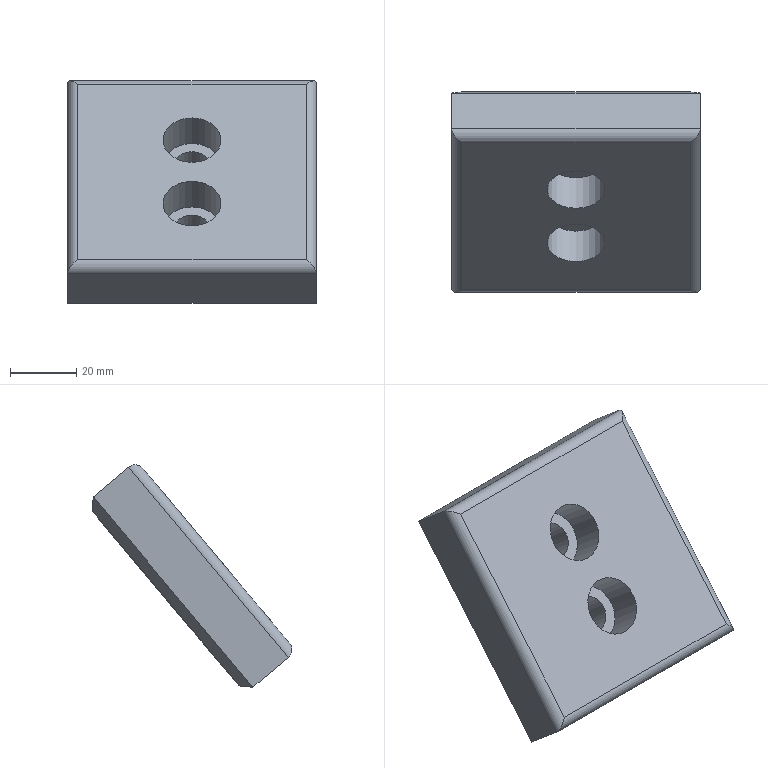Part | NX | features solid 2 | 1 solid | 20 faces | box 75 x 60.375 x 67.154 mm | volume 103324 mm3 | plane 12 | cylinder 8 | commonest cylinder face diameters 6 x4 11 x2 17.5 x2
STEP:
#1=CARTESIAN_POINT('',(432.5,190.843,-55.704));
#2=VERTEX_POINT('',#1);
#3=CARTESIAN_POINT('',(432.5,180.118,-46.705));
#4=VERTEX_POINT('',#3);
#5=CARTESIAN_POINT('',(432.5,193.141,-57.632));
#6=DIRECTION('',(0.,-0.766,0.6428));
#7=VECTOR('',#6,1000.);
#8=LINE('',#5,#7);
#9=EDGE_CURVE('',#2,#4,#8,.T.);
#10=ORIENTED_EDGE('',*,*,#9,.T.);
#11=CARTESIAN_POINT('',(357.5,180.118,-46.705));
#12=VERTEX_POINT('',#11);
#13=CARTESIAN_POINT('',(432.5,180.118,-46.705));
#14=DIRECTION('',(1.,0.,0.));
#15=VECTOR('',#14,1000.);
#16=LINE('',#13,#15);
#17=EDGE_CURVE('',#12,#4,#16,.T.);
#18=ORIENTED_EDGE('',*,*,#17,.F.);
#19=CARTESIAN_POINT('',(357.5,190.843,-55.704));
#20=VERTEX_POINT('',#19);
#21=CARTESIAN_POINT('',(357.5,193.141,-57.632));
#22=DIRECTION('',(0.,-0.766,0.6428));
#23=VECTOR('',#22,1000.);
#24=LINE('',#21,#23);
#25=EDGE_CURVE('',#20,#12,#24,.T.);
#26=ORIENTED_EDGE('',*,*,#25,.F.);
#27=CARTESIAN_POINT('',(357.5,190.843,-55.704));
#28=DIRECTION('',(-1.,0.,0.));
#29=VECTOR('',#28,1000.);
#30=LINE('',#27,#29);
#31=EDGE_CURVE('',#2,#20,#30,.T.);
#32=ORIENTED_EDGE('',*,*,#31,.F.);
#33=EDGE_LOOP('',(#10,#18,#26,#32));
#34=FACE_BOUND('',#33,.T.);
#35=CARTESIAN_POINT('',(357.5,193.141,-57.632));
#36=DIRECTION('',(0.,0.6428,0.766));
#37=DIRECTION('',(-1.,0.,0.));
#38=AXIS2_PLACEMENT_3D('',#35,#36,#37);
#39=PLANE('',#38);
#40=ADVANCED_FACE('',(#34),#39,.F.);
#41=CARTESIAN_POINT('',(432.5,239.052,1.75));
#42=VERTEX_POINT('',#41);
#43=CARTESIAN_POINT('',(432.5,228.328,10.749));
#44=VERTEX_POINT('',#43);
#45=CARTESIAN_POINT('',(432.5,241.35,-0.1788));
#46=DIRECTION('',(0.,-0.766,0.6428));
#47=VECTOR('',#46,1000.);
#48=LINE('',#45,#47);
#49=EDGE_CURVE('',#42,#44,#48,.T.);
#50=ORIENTED_EDGE('',*,*,#49,.T.);
#51=CARTESIAN_POINT('',(432.5,244.397,29.9));
#52=DIRECTION('',(0.,0.6428,0.766));
#53=VECTOR('',#52,1000.);
#54=LINE('',#51,#53);
#55=EDGE_CURVE('',#4,#44,#54,.T.);
#56=ORIENTED_EDGE('',*,*,#55,.F.);
#57=ORIENTED_EDGE('',*,*,#9,.F.);
#58=CARTESIAN_POINT('',(432.5,190.843,-55.704));
#59=DIRECTION('',(0.,-0.6428,-0.766));
#60=VECTOR('',#59,1000.);
#61=LINE('',#58,#60);
#62=EDGE_CURVE('',#42,#2,#61,.T.);
#63=ORIENTED_EDGE('',*,*,#62,.F.);
#64=EDGE_LOOP('',(#50,#56,#57,#63));
#65=FACE_BOUND('',#64,.T.);
#66=CARTESIAN_POINT('',(432.5,193.141,-57.632));
#67=DIRECTION('',(-1.,0.,0.));
#68=DIRECTION('',(0.,0.766,-0.6428));
#69=AXIS2_PLACEMENT_3D('',#66,#67,#68);
#70=PLANE('',#69);
#71=ADVANCED_FACE('',(#65),#70,.F.);
#72=CARTESIAN_POINT('',(357.5,239.052,1.75));
#73=VERTEX_POINT('',#72);
#74=CARTESIAN_POINT('',(357.5,228.328,10.749));
#75=VERTEX_POINT('',#74);
#76=CARTESIAN_POINT('',(357.5,241.35,-0.1788));
#77=DIRECTION('',(0.,-0.766,0.6428));
#78=VECTOR('',#77,1000.);
#79=LINE('',#76,#78);
#80=EDGE_CURVE('',#73,#75,#79,.T.);
#81=ORIENTED_EDGE('',*,*,#80,.T.);
#82=CARTESIAN_POINT('',(357.5,228.328,10.749));
#83=DIRECTION('',(-1.,0.,0.));
#84=VECTOR('',#83,1000.);
#85=LINE('',#82,#84);
#86=EDGE_CURVE('',#44,#75,#85,.T.);
#87=ORIENTED_EDGE('',*,*,#86,.F.);
#88=ORIENTED_EDGE('',*,*,#49,.F.);
#89=CARTESIAN_POINT('',(432.5,239.052,1.75));
#90=DIRECTION('',(1.,0.,0.));
#91=VECTOR('',#90,1000.);
#92=LINE('',#89,#91);
#93=EDGE_CURVE('',#73,#42,#92,.T.);
#94=ORIENTED_EDGE('',*,*,#93,.F.);
#95=EDGE_LOOP('',(#81,#87,#88,#94));
#96=FACE_BOUND('',#95,.T.);
#97=CARTESIAN_POINT('',(432.5,241.35,-0.1788));
#98=DIRECTION('',(0.,-0.6428,-0.766));
#99=DIRECTION('',(0.,0.766,-0.6428));
#100=AXIS2_PLACEMENT_3D('',#97,#98,#99);
#101=PLANE('',#100);
#102=ADVANCED_FACE('',(#96),#101,.F.);
#103=ORIENTED_EDGE('',*,*,#25,.T.);
#104=CARTESIAN_POINT('',(357.5,180.118,-46.705));
#105=DIRECTION('',(0.,-0.6428,-0.766));
#106=VECTOR('',#105,1000.);
#107=LINE('',#104,#106);
#108=EDGE_CURVE('',#75,#12,#107,.T.);
#109=ORIENTED_EDGE('',*,*,#108,.F.);
#110=ORIENTED_EDGE('',*,*,#80,.F.);
#111=CARTESIAN_POINT('',(357.5,255.122,20.901));
#112=DIRECTION('',(0.,0.6428,0.766));
#113=VECTOR('',#112,1000.);
#114=LINE('',#111,#113);
#115=EDGE_CURVE('',#20,#73,#114,.T.);
#116=ORIENTED_EDGE('',*,*,#115,.F.);
#117=EDGE_LOOP('',(#103,#109,#110,#116));
#118=FACE_BOUND('',#117,.T.);
#119=CARTESIAN_POINT('',(357.5,257.42,18.972));
#120=DIRECTION('',(1.,0.,0.));
#121=DIRECTION('',(0.,0.6428,0.766));
#122=AXIS2_PLACEMENT_3D('',#119,#120,#121);
#123=PLANE('',#122);
#124=ADVANCED_FACE('',(#118),#123,.F.);
#125=CARTESIAN_POINT('',(429.5,195.07,-55.334));
#126=VERTEX_POINT('',#125);
#127=CARTESIAN_POINT('',(429.5,239.422,-2.477));
#128=VERTEX_POINT('',#127);
#129=CARTESIAN_POINT('',(429.5,193.141,-57.632));
#130=DIRECTION('',(0.,0.6428,0.766));
#131=VECTOR('',#130,1000.);
#132=LINE('',#129,#131);
#133=EDGE_CURVE('',#126,#128,#132,.T.);
#134=ORIENTED_EDGE('',*,*,#133,.F.);
#135=CARTESIAN_POINT('',(360.5,195.07,-55.334));
#136=VERTEX_POINT('',#135);
#137=CARTESIAN_POINT('',(357.5,195.07,-55.334));
#138=DIRECTION('',(1.,0.,0.));
#139=VECTOR('',#138,1000.);
#140=LINE('',#137,#139);
#141=EDGE_CURVE('',#136,#126,#140,.T.);
#142=ORIENTED_EDGE('',*,*,#141,.F.);
#143=CARTESIAN_POINT('',(360.5,239.422,-2.477));
#144=VERTEX_POINT('',#143);
#145=CARTESIAN_POINT('',(360.5,193.141,-57.632));
#146=DIRECTION('',(0.,-0.6428,-0.766));
#147=VECTOR('',#146,1000.);
#148=LINE('',#145,#147);
#149=EDGE_CURVE('',#144,#136,#148,.T.);
#150=ORIENTED_EDGE('',*,*,#149,.F.);
#151=CARTESIAN_POINT('',(357.5,239.422,-2.477));
#152=DIRECTION('',(-1.,0.,0.));
#153=VECTOR('',#152,1000.);
#154=LINE('',#151,#153);
#155=EDGE_CURVE('',#128,#144,#154,.T.);
#156=ORIENTED_EDGE('',*,*,#155,.F.);
#157=EDGE_LOOP('',(#134,#142,#150,#156));
#158=FACE_BOUND('',#157,.T.);
#159=CARTESIAN_POINT('',(395.,221.745,-23.543));
#160=VERTEX_POINT('',#159);
#161=CARTESIAN_POINT('',(395.,225.281,-19.33));
#162=DIRECTION('',(0.,0.766,-0.6428));
#163=DIRECTION('',(0.,-0.6428,-0.766));
#164=AXIS2_PLACEMENT_3D('',#161,#162,#163);
#165=CIRCLE('',#164,5.5);
#166=EDGE_CURVE('',#160,#160,#165,.T.);
#167=ORIENTED_EDGE('',*,*,#166,.F.);
#168=EDGE_LOOP('',(#167));
#169=FACE_BOUND('',#168,.T.);
#170=CARTESIAN_POINT('',(395.,205.676,-42.694));
#171=VERTEX_POINT('',#170);
#172=CARTESIAN_POINT('',(395.,209.211,-38.481));
#173=DIRECTION('',(0.,0.766,-0.6428));
#174=DIRECTION('',(0.,-0.6428,-0.766));
#175=AXIS2_PLACEMENT_3D('',#172,#173,#174);
#176=CIRCLE('',#175,5.5);
#177=EDGE_CURVE('',#171,#171,#176,.T.);
#178=ORIENTED_EDGE('',*,*,#177,.F.);
#179=EDGE_LOOP('',(#178));
#180=FACE_BOUND('',#179,.T.);
#181=CARTESIAN_POINT('',(357.5,193.141,-57.632));
#182=DIRECTION('',(0.,-0.766,0.6428));
#183=DIRECTION('',(0.,-0.6428,-0.766));
#184=AXIS2_PLACEMENT_3D('',#181,#182,#183);
#185=PLANE('',#184);
#186=ADVANCED_FACE('',(#158,#169,#180),#185,.F.);
#187=CARTESIAN_POINT('',(429.5,179.749,-42.478));
#188=VERTEX_POINT('',#187);
#189=CARTESIAN_POINT('',(360.5,179.749,-42.478));
#190=VERTEX_POINT('',#189);
#191=CARTESIAN_POINT('',(357.5,179.749,-42.478));
#192=DIRECTION('',(1.,0.,0.));
#193=VECTOR('',#192,1000.);
#194=LINE('',#191,#193);
#195=EDGE_CURVE('',#188,#190,#194,.F.);
#196=ORIENTED_EDGE('',*,*,#195,.F.);
#197=CARTESIAN_POINT('',(429.5,224.101,10.379));
#198=VERTEX_POINT('',#197);
#199=CARTESIAN_POINT('',(429.5,177.82,-44.776));
#200=DIRECTION('',(0.,0.6428,0.766));
#201=VECTOR('',#200,1000.);
#202=LINE('',#199,#201);
#203=EDGE_CURVE('',#198,#188,#202,.F.);
#204=ORIENTED_EDGE('',*,*,#203,.F.);
#205=CARTESIAN_POINT('',(360.5,224.101,10.379));
#206=VERTEX_POINT('',#205);
#207=CARTESIAN_POINT('',(432.5,224.101,10.379));
#208=DIRECTION('',(-1.,0.,0.));
#209=VECTOR('',#208,1000.);
#210=LINE('',#207,#209);
#211=EDGE_CURVE('',#206,#198,#210,.F.);
#212=ORIENTED_EDGE('',*,*,#211,.F.);
#213=CARTESIAN_POINT('',(360.5,242.099,31.828));
#214=DIRECTION('',(0.,-0.6428,-0.766));
#215=VECTOR('',#214,1000.);
#216=LINE('',#213,#215);
#217=EDGE_CURVE('',#190,#206,#216,.F.);
#218=ORIENTED_EDGE('',*,*,#217,.F.);
#219=EDGE_LOOP('',(#196,#204,#212,#218));
#220=FACE_BOUND('',#219,.T.);
#221=CARTESIAN_POINT('',(395.,215.584,0.2287));
#222=VERTEX_POINT('',#221);
#223=CARTESIAN_POINT('',(395.,209.96,-6.474));
#224=DIRECTION('',(0.,-0.766,0.6428));
#225=DIRECTION('',(0.,0.6428,0.766));
#226=AXIS2_PLACEMENT_3D('',#223,#224,#225);
#227=CIRCLE('',#226,8.75);
#228=EDGE_CURVE('',#222,#222,#227,.T.);
#229=ORIENTED_EDGE('',*,*,#228,.F.);
#230=EDGE_LOOP('',(#229));
#231=FACE_BOUND('',#230,.T.);
#232=CARTESIAN_POINT('',(395.,199.514,-18.922));
#233=VERTEX_POINT('',#232);
#234=CARTESIAN_POINT('',(395.,193.89,-25.625));
#235=DIRECTION('',(0.,-0.766,0.6428));
#236=DIRECTION('',(0.,0.6428,0.766));
#237=AXIS2_PLACEMENT_3D('',#234,#235,#236);
#238=CIRCLE('',#237,8.75);
#239=EDGE_CURVE('',#233,#233,#238,.T.);
#240=ORIENTED_EDGE('',*,*,#239,.F.);
#241=EDGE_LOOP('',(#240));
#242=FACE_BOUND('',#241,.T.);
#243=CARTESIAN_POINT('',(357.5,177.82,-44.776));
#244=DIRECTION('',(0.,-0.766,0.6428));
#245=DIRECTION('',(0.,-0.6428,-0.766));
#246=AXIS2_PLACEMENT_3D('',#243,#244,#245);
#247=PLANE('',#246);
#248=ADVANCED_FACE('',(#220,#231,#242),#247,.T.);
#249=CARTESIAN_POINT('',(395.,206.618,-29.125));
#250=VERTEX_POINT('',#249);
#251=CARTESIAN_POINT('',(395.,203.083,-33.339));
#252=DIRECTION('',(0.,-0.766,0.6428));
#253=DIRECTION('',(0.,0.6428,0.766));
#254=AXIS2_PLACEMENT_3D('',#251,#252,#253);
#255=CIRCLE('',#254,5.5);
#256=EDGE_CURVE('',#250,#250,#255,.T.);
#257=ORIENTED_EDGE('',*,*,#256,.T.);
#258=EDGE_LOOP('',(#257));
#259=FACE_BOUND('',#258,.T.);
#260=ORIENTED_EDGE('',*,*,#177,.T.);
#261=EDGE_LOOP('',(#260));
#262=FACE_BOUND('',#261,.T.);
#263=CARTESIAN_POINT('',(395.,232.192,-57.765));
#264=DIRECTION('',(0.,0.766,-0.6428));
#265=DIRECTION('',(0.,0.6428,0.766));
#266=AXIS2_PLACEMENT_3D('',#263,#264,#265);
#267=CYLINDRICAL_SURFACE('',#266,5.5);
#268=ADVANCED_FACE('',(#259,#262),#267,.F.);
#269=ORIENTED_EDGE('',*,*,#256,.F.);
#270=EDGE_LOOP('',(#269));
#271=FACE_BOUND('',#270,.T.);
#272=CARTESIAN_POINT('',(395.,208.707,-26.636));
#273=VERTEX_POINT('',#272);
#274=CARTESIAN_POINT('',(395.,203.083,-33.339));
#275=DIRECTION('',(0.,-0.766,0.6428));
#276=DIRECTION('',(0.,0.6428,0.766));
#277=AXIS2_PLACEMENT_3D('',#274,#275,#276);
#278=CIRCLE('',#277,8.75);
#279=EDGE_CURVE('',#273,#273,#278,.T.);
#280=ORIENTED_EDGE('',*,*,#279,.T.);
#281=EDGE_LOOP('',(#280));
#282=FACE_BOUND('',#281,.T.);
#283=CARTESIAN_POINT('',(395.,203.083,-33.339));
#284=DIRECTION('',(0.,0.766,-0.6428));
#285=DIRECTION('',(0.,0.6428,0.766));
#286=AXIS2_PLACEMENT_3D('',#283,#284,#285);
#287=PLANE('',#286);
#288=ADVANCED_FACE('',(#271,#282),#287,.F.);
#289=ORIENTED_EDGE('',*,*,#279,.F.);
#290=EDGE_LOOP('',(#289));
#291=FACE_BOUND('',#290,.T.);
#292=ORIENTED_EDGE('',*,*,#239,.T.);
#293=EDGE_LOOP('',(#292));
#294=FACE_BOUND('',#293,.T.);
#295=CARTESIAN_POINT('',(395.,193.89,-25.625));
#296=DIRECTION('',(0.,0.766,-0.6428));
#297=DIRECTION('',(0.,0.6428,0.766));
#298=AXIS2_PLACEMENT_3D('',#295,#296,#297);
#299=CYLINDRICAL_SURFACE('',#298,8.75);
#300=ADVANCED_FACE('',(#291,#294),#299,.F.);
#301=CARTESIAN_POINT('',(395.,222.688,-9.974));
#302=VERTEX_POINT('',#301);
#303=CARTESIAN_POINT('',(395.,219.152,-14.188));
#304=DIRECTION('',(0.,-0.766,0.6428));
#305=DIRECTION('',(0.,0.6428,0.766));
#306=AXIS2_PLACEMENT_3D('',#303,#304,#305);
#307=CIRCLE('',#306,5.5);
#308=EDGE_CURVE('',#302,#302,#307,.T.);
#309=ORIENTED_EDGE('',*,*,#308,.T.);
#310=EDGE_LOOP('',(#309));
#311=FACE_BOUND('',#310,.T.);
#312=ORIENTED_EDGE('',*,*,#166,.T.);
#313=EDGE_LOOP('',(#312));
#314=FACE_BOUND('',#313,.T.);
#315=CARTESIAN_POINT('',(395.,248.262,-38.614));
#316=DIRECTION('',(0.,0.766,-0.6428));
#317=DIRECTION('',(0.,0.6428,0.766));
#318=AXIS2_PLACEMENT_3D('',#315,#316,#317);
#319=CYLINDRICAL_SURFACE('',#318,5.5);
#320=ADVANCED_FACE('',(#311,#314),#319,.F.);
#321=ORIENTED_EDGE('',*,*,#308,.F.);
#322=EDGE_LOOP('',(#321));
#323=FACE_BOUND('',#322,.T.);
#324=CARTESIAN_POINT('',(395.,224.777,-7.485));
#325=VERTEX_POINT('',#324);
#326=CARTESIAN_POINT('',(395.,219.152,-14.188));
#327=DIRECTION('',(0.,-0.766,0.6428));
#328=DIRECTION('',(0.,0.6428,0.766));
#329=AXIS2_PLACEMENT_3D('',#326,#327,#328);
#330=CIRCLE('',#329,8.75);
#331=EDGE_CURVE('',#325,#325,#330,.T.);
#332=ORIENTED_EDGE('',*,*,#331,.T.);
#333=EDGE_LOOP('',(#332));
#334=FACE_BOUND('',#333,.T.);
#335=CARTESIAN_POINT('',(395.,219.152,-14.188));
#336=DIRECTION('',(0.,0.766,-0.6428));
#337=DIRECTION('',(0.,0.6428,0.766));
#338=AXIS2_PLACEMENT_3D('',#335,#336,#337);
#339=PLANE('',#338);
#340=ADVANCED_FACE('',(#323,#334),#339,.F.);
#341=ORIENTED_EDGE('',*,*,#331,.F.);
#342=EDGE_LOOP('',(#341));
#343=FACE_BOUND('',#342,.T.);
#344=ORIENTED_EDGE('',*,*,#228,.T.);
#345=EDGE_LOOP('',(#344));
#346=FACE_BOUND('',#345,.T.);
#347=CARTESIAN_POINT('',(395.,209.96,-6.474));
#348=DIRECTION('',(0.,0.766,-0.6428));
#349=DIRECTION('',(0.,0.6428,0.766));
#350=AXIS2_PLACEMENT_3D('',#347,#348,#349);
#351=CYLINDRICAL_SURFACE('',#350,8.75);
#352=ADVANCED_FACE('',(#343,#346),#351,.F.);
#353=CARTESIAN_POINT('',(429.5,182.047,-44.407));
#354=DIRECTION('',(0.7071,0.4545,0.5417));
#355=DIRECTION('',(-0.7071,0.4545,0.5417));
#356=AXIS2_PLACEMENT_3D('',#353,#354,#355);
#357=ELLIPSE('',#356,4.243,3.);
#358=EDGE_CURVE('',#188,#4,#357,.T.);
#359=ORIENTED_EDGE('',*,*,#358,.T.);
#360=ORIENTED_EDGE('',*,*,#55,.T.);
#361=CARTESIAN_POINT('',(429.5,226.399,8.45));
#362=DIRECTION('',(-0.7071,0.4545,0.5417));
#363=DIRECTION('',(-0.7071,-0.4545,-0.5417));
#364=AXIS2_PLACEMENT_3D('',#361,#362,#363);
#365=ELLIPSE('',#364,4.243,3.);
#366=EDGE_CURVE('',#44,#198,#365,.F.);
#367=ORIENTED_EDGE('',*,*,#366,.T.);
#368=ORIENTED_EDGE('',*,*,#203,.T.);
#369=EDGE_LOOP('',(#359,#360,#367,#368));
#370=FACE_BOUND('',#369,.T.);
#371=CARTESIAN_POINT('',(429.5,180.118,-46.705));
#372=DIRECTION('',(0.,-0.6428,-0.766));
#373=DIRECTION('',(0.,0.766,-0.6428));
#374=AXIS2_PLACEMENT_3D('',#371,#372,#373);
#375=CYLINDRICAL_SURFACE('',#374,3.);
#376=ADVANCED_FACE('',(#370),#375,.T.);
#377=ORIENTED_EDGE('',*,*,#366,.F.);
#378=ORIENTED_EDGE('',*,*,#86,.T.);
#379=CARTESIAN_POINT('',(360.5,226.399,8.45));
#380=DIRECTION('',(-0.7071,-0.4545,-0.5417));
#381=DIRECTION('',(0.7071,-0.4545,-0.5417));
#382=AXIS2_PLACEMENT_3D('',#379,#380,#381);
#383=ELLIPSE('',#382,4.243,3.);
#384=EDGE_CURVE('',#75,#206,#383,.F.);
#385=ORIENTED_EDGE('',*,*,#384,.T.);
#386=ORIENTED_EDGE('',*,*,#211,.T.);
#387=EDGE_LOOP('',(#377,#378,#385,#386));
#388=FACE_BOUND('',#387,.T.);
#389=CARTESIAN_POINT('',(432.5,226.399,8.45));
#390=DIRECTION('',(1.,0.,0.));
#391=DIRECTION('',(0.,-0.766,0.6428));
#392=AXIS2_PLACEMENT_3D('',#389,#390,#391);
#393=CYLINDRICAL_SURFACE('',#392,3.);
#394=ADVANCED_FACE('',(#388),#393,.T.);
#395=ORIENTED_EDGE('',*,*,#358,.F.);
#396=ORIENTED_EDGE('',*,*,#195,.T.);
#397=CARTESIAN_POINT('',(360.5,182.047,-44.407));
#398=DIRECTION('',(0.7071,-0.4545,-0.5417));
#399=DIRECTION('',(-0.7071,-0.4545,-0.5417));
#400=AXIS2_PLACEMENT_3D('',#397,#398,#399);
#401=ELLIPSE('',#400,4.243,3.);
#402=EDGE_CURVE('',#190,#12,#401,.T.);
#403=ORIENTED_EDGE('',*,*,#402,.T.);
#404=ORIENTED_EDGE('',*,*,#17,.T.);
#405=EDGE_LOOP('',(#395,#396,#403,#404));
#406=FACE_BOUND('',#405,.T.);
#407=CARTESIAN_POINT('',(357.5,182.047,-44.407));
#408=DIRECTION('',(-1.,0.,0.));
#409=DIRECTION('',(0.,-0.6428,-0.766));
#410=AXIS2_PLACEMENT_3D('',#407,#408,#409);
#411=CYLINDRICAL_SURFACE('',#410,3.);
#412=ADVANCED_FACE('',(#406),#411,.T.);
#413=ORIENTED_EDGE('',*,*,#384,.F.);
#414=ORIENTED_EDGE('',*,*,#108,.T.);
#415=ORIENTED_EDGE('',*,*,#402,.F.);
#416=ORIENTED_EDGE('',*,*,#217,.T.);
#417=EDGE_LOOP('',(#413,#414,#415,#416));
#418=FACE_BOUND('',#417,.T.);
#419=CARTESIAN_POINT('',(360.5,244.397,29.9));
#420=DIRECTION('',(0.,0.6428,0.766));
#421=DIRECTION('',(-1.,0.,0.));
#422=AXIS2_PLACEMENT_3D('',#419,#420,#421);
#423=CYLINDRICAL_SURFACE('',#422,3.);
#424=ADVANCED_FACE('',(#418),#423,.T.);
#425=CARTESIAN_POINT('',(359.5,193.661,-55.457));
#426=DIRECTION('',(0.5774,0.8134,0.07116));
#427=VECTOR('',#426,1000.);
#428=LINE('',#425,#427);
#429=EDGE_CURVE('',#20,#136,#428,.T.);
#430=ORIENTED_EDGE('',*,*,#429,.T.);
#431=ORIENTED_EDGE('',*,*,#141,.T.);
#432=CARTESIAN_POINT('',(405.5,228.882,-52.376));
#433=DIRECTION('',(-0.5774,0.8134,0.07116));
#434=VECTOR('',#433,1000.);
#435=LINE('',#432,#434);
#436=EDGE_CURVE('',#126,#2,#435,.F.);
#437=ORIENTED_EDGE('',*,*,#436,.T.);
#438=ORIENTED_EDGE('',*,*,#31,.T.);
#439=EDGE_LOOP('',(#430,#431,#437,#438));
#440=FACE_BOUND('',#439,.T.);
#441=CARTESIAN_POINT('',(357.5,195.07,-55.334));
#442=DIRECTION('',(0.,-0.08716,0.9962));
#443=DIRECTION('',(0.,-0.9962,-0.08716));
#444=AXIS2_PLACEMENT_3D('',#441,#442,#443);
#445=PLANE('',#444);
#446=ADVANCED_FACE('',(#440),#445,.F.);
#447=ORIENTED_EDGE('',*,*,#436,.F.);
#448=ORIENTED_EDGE('',*,*,#133,.T.);
#449=CARTESIAN_POINT('',(397.167,243.407,-48.029));
#450=DIRECTION('',(-0.5774,0.07116,-0.8134));
#451=VECTOR('',#450,1000.);
#452=LINE('',#449,#451);
#453=EDGE_CURVE('',#128,#42,#452,.F.);
#454=ORIENTED_EDGE('',*,*,#453,.T.);
#455=ORIENTED_EDGE('',*,*,#62,.T.);
#456=EDGE_LOOP('',(#447,#448,#454,#455));
#457=FACE_BOUND('',#456,.T.);
#458=CARTESIAN_POINT('',(429.5,193.141,-57.632));
#459=DIRECTION('',(-0.7071,-0.5417,0.4545));
#460=DIRECTION('',(-0.7071,0.5417,-0.4545));
#461=AXIS2_PLACEMENT_3D('',#458,#459,#460);
#462=PLANE('',#461);
#463=ADVANCED_FACE('',(#457),#462,.F.);
#464=ORIENTED_EDGE('',*,*,#429,.F.);
#465=ORIENTED_EDGE('',*,*,#115,.T.);
#466=CARTESIAN_POINT('',(392.833,243.407,-48.029));
#467=DIRECTION('',(-0.5774,-0.07116,0.8134));
#468=VECTOR('',#467,1000.);
#469=LINE('',#466,#468);
#470=EDGE_CURVE('',#73,#144,#469,.F.);
#471=ORIENTED_EDGE('',*,*,#470,.T.);
#472=ORIENTED_EDGE('',*,*,#149,.T.);
#473=EDGE_LOOP('',(#464,#465,#471,#472));
#474=FACE_BOUND('',#473,.T.);
#475=CARTESIAN_POINT('',(360.5,193.141,-57.632));
#476=DIRECTION('',(0.7071,-0.5417,0.4545));
#477=DIRECTION('',(-0.7071,-0.5417,0.4545));
#478=AXIS2_PLACEMENT_3D('',#475,#476,#477);
#479=PLANE('',#478);
#480=ADVANCED_FACE('',(#474),#479,.F.);
#481=ORIENTED_EDGE('',*,*,#453,.F.);
#482=ORIENTED_EDGE('',*,*,#155,.T.);
#483=ORIENTED_EDGE('',*,*,#470,.F.);
#484=ORIENTED_EDGE('',*,*,#93,.T.);
#485=EDGE_LOOP('',(#481,#482,#483,#484));
#486=FACE_BOUND('',#485,.T.);
#487=CARTESIAN_POINT('',(357.5,239.422,-2.477));
#488=DIRECTION('',(0.,-0.9962,-0.08716));
#489=DIRECTION('',(0.,0.08716,-0.9962));
#490=AXIS2_PLACEMENT_3D('',#487,#488,#489);
#491=PLANE('',#490);
#492=ADVANCED_FACE('',(#486),#491,.F.);
#493=CLOSED_SHELL('',(#40,#71,#102,#124,#186,#248,#268,#288,#300,#320,#340,#352,#376,#394,#412,#424,#446,#463,#480,#492));
#494=MANIFOLD_SOLID_BREP('',#493);
#495=(LENGTH_UNIT()NAMED_UNIT(*)SI_UNIT(.MILLI.,.METRE.));
#496=UNCERTAINTY_MEASURE_WITH_UNIT(LENGTH_MEASURE(0.00001),#495,'','');
#497=(NAMED_UNIT(*)PLANE_ANGLE_UNIT()SI_UNIT($,.RADIAN.));
#498=(NAMED_UNIT(*)SI_UNIT($,.STERADIAN.)SOLID_ANGLE_UNIT());
#499=(GEOMETRIC_REPRESENTATION_CONTEXT(3)GLOBAL_UNCERTAINTY_ASSIGNED_CONTEXT((#496))GLOBAL_UNIT_ASSIGNED_CONTEXT((#495,#497,#498))REPRESENTATION_CONTEXT('',''));
#500=ADVANCED_BREP_SHAPE_REPRESENTATION('',(#494),#499);